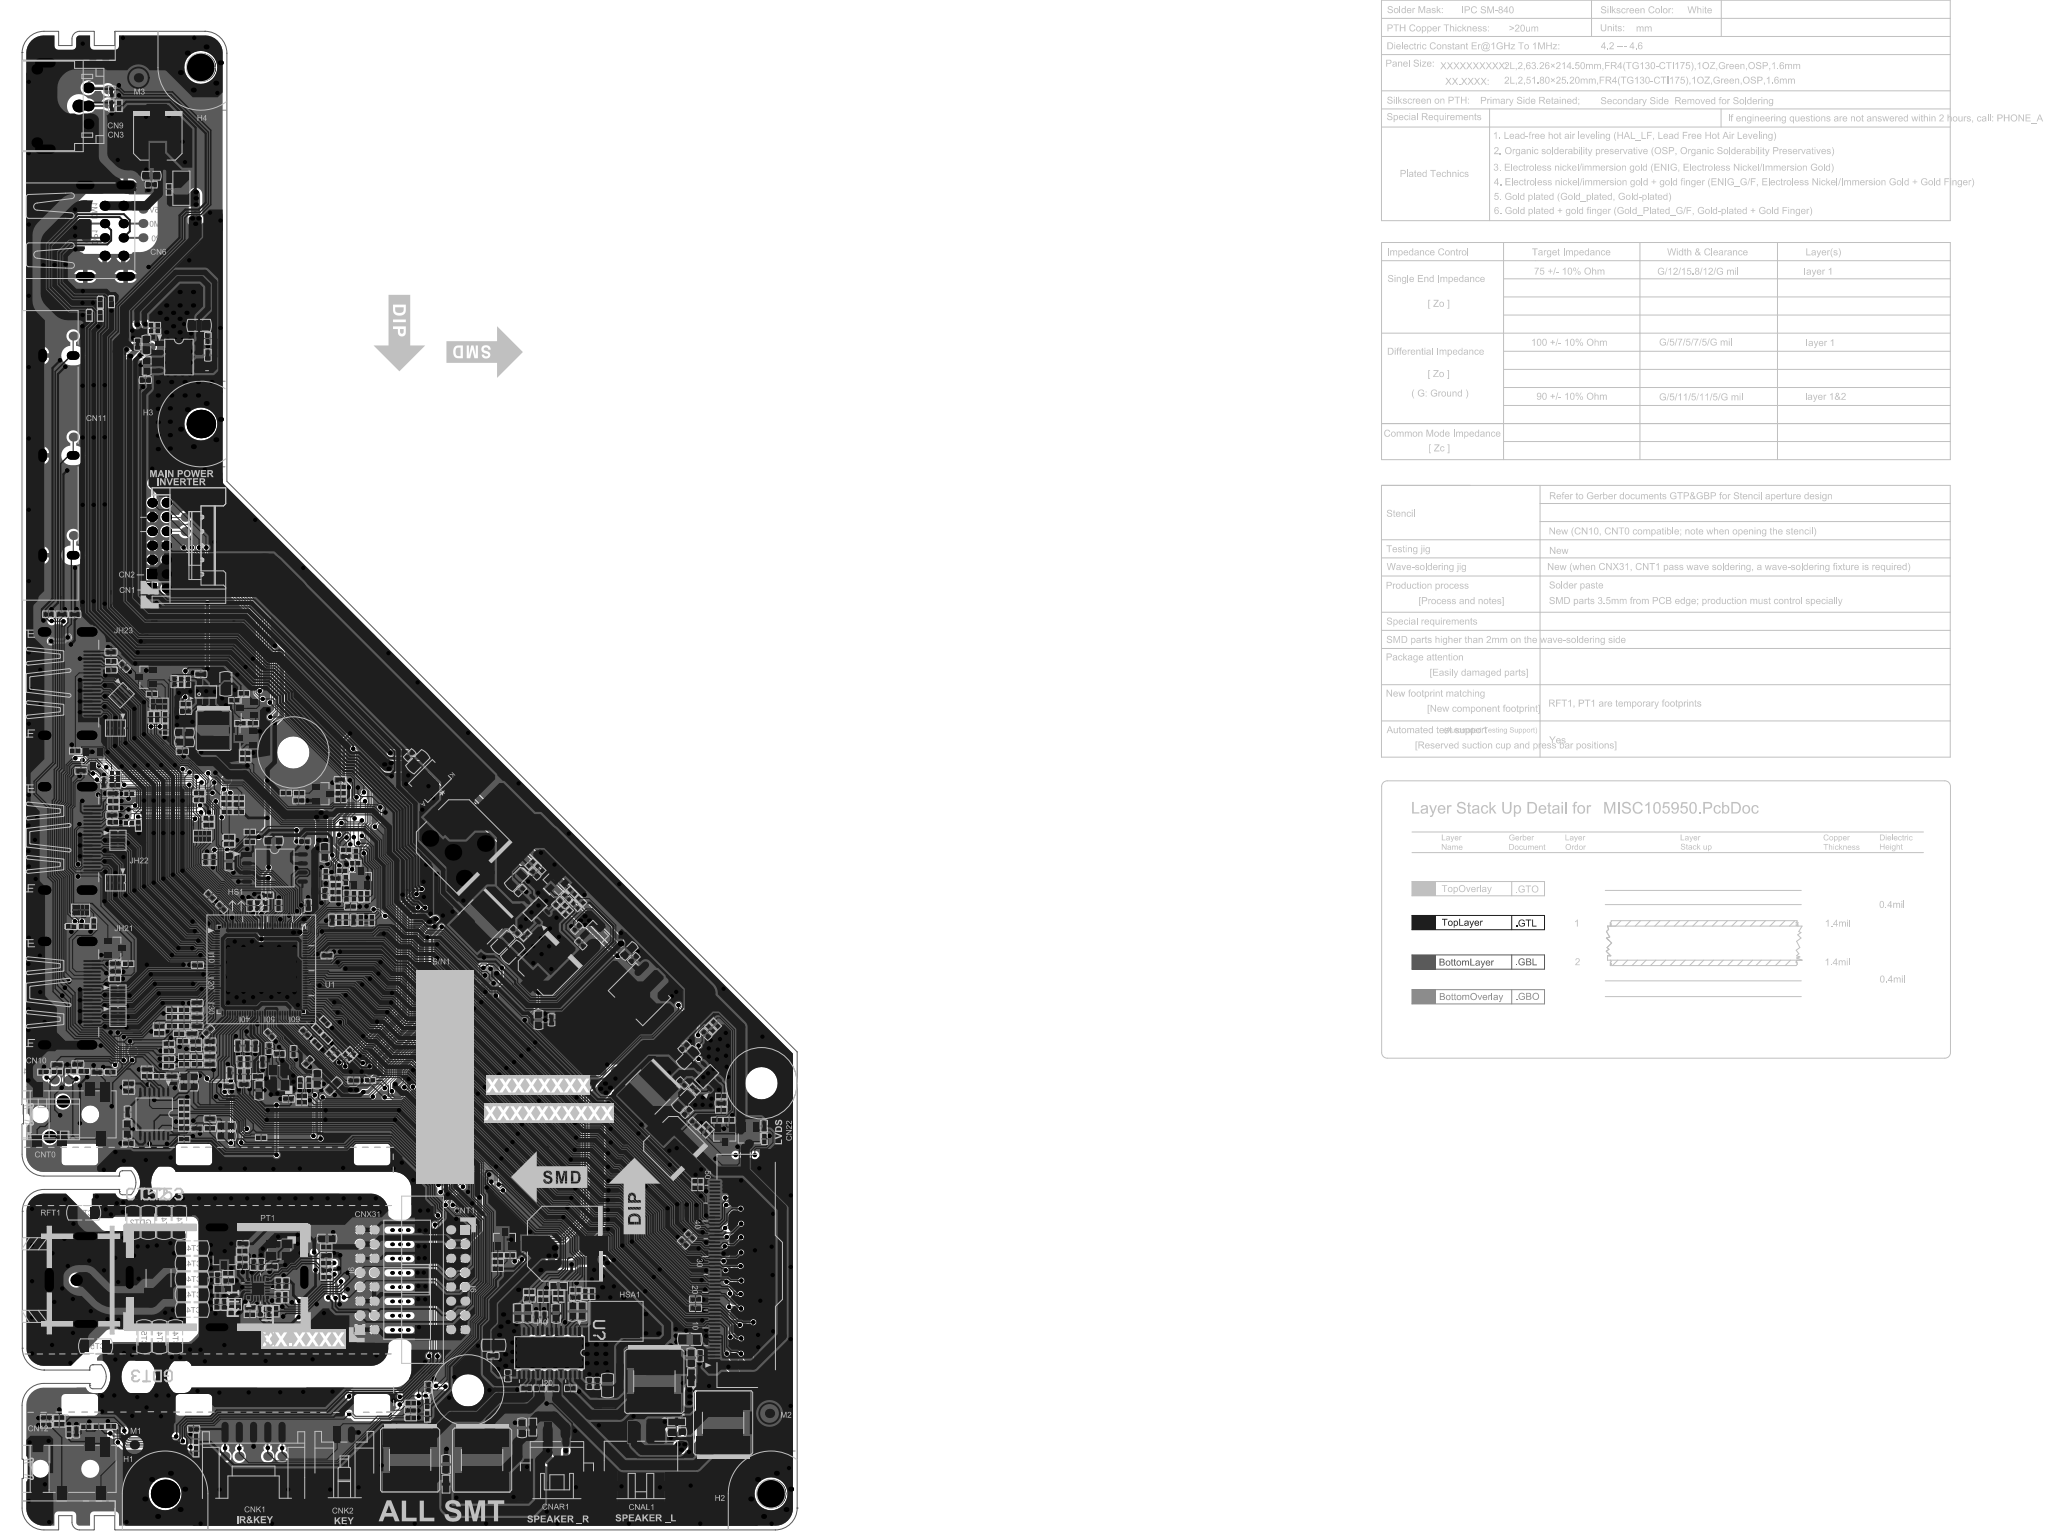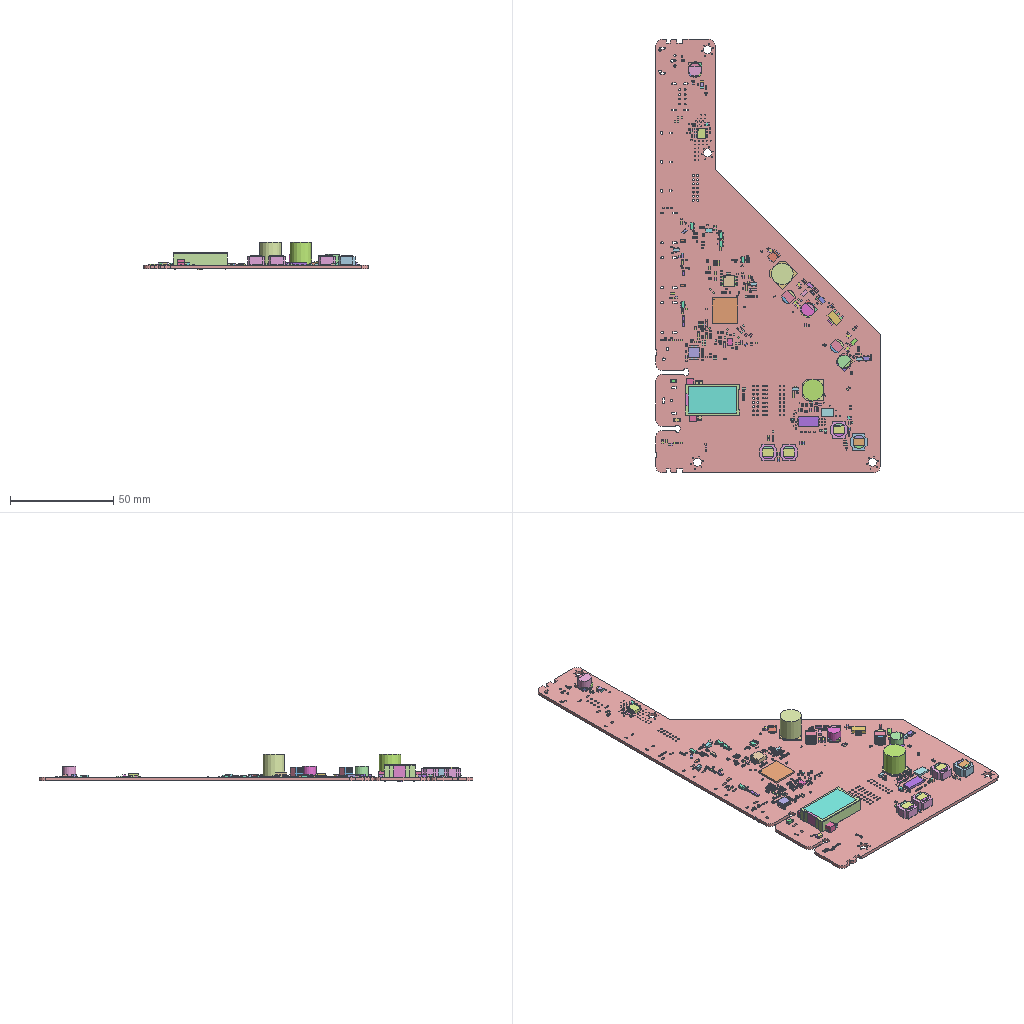Circuit board layout | Altium Designer | box 108.7 x 210.1 x 13.1 mm
Layer stack:
# Altium Designer layer stack of  (unit mm; dielectric type: 0 none, 1 core, 2 prepreg, 3 surface material)
index,name,kind,layer,copper_thickness_mm,dielectric_type,dielectric_thickness_mm,dielectric_material,dielectric_constant
0,TopPaste,other,,,,,,
1,TopOverlay,other,,,,,,
2,TopSolder,dielectric,,,3,0.0102,Solder Resist,3.5
3,TopLayer,copper,TopLayer,0.0356,,,,
4,Dielectric1,dielectric,,,1,1.5,FR-4,4.8
5,BottomLayer,copper,BottomLayer,0.0356,,,,
6,BottomSolder,dielectric,,,3,0.0102,Solder Resist,3.5
7,BottomOverlay,other,,,,,,
8,BottomPaste,other,,,,,,
# drill layer pairs: low layer,high layer
drill_pair,TopLayer,BottomLayer
Part placement, first 366 of 542 lines:
Designator,Comment,Layer,Footprint,Center-X(mm),Center-Y(mm),Rotation
YPbPr_Pb,TEST,BottomLayer,TP,6.464,63.03,180
DI33,NC/SFI0402-240E-2R5PP-LF,TopLayer,DIODE-S0402,20.485,64.935,360
DU31,NC/TVS diode, DIO ESD, 0.1pF, 25V, 0402, SMD, GESD1005H150CR10GPT, Sunlord,TopLayer,DIODE-S0402,41.391,70.115,315
RD66,NC/0ohm-0402-PCB,TopLayer,R0402SC,70.561,83.299,45
RD65,NC/0ohm-0402-PCB,TopLayer,R0402SC,94.272,61.735,315
DU34,NC/TVS diode, DIO ESD, 0.1pF, 25V, 0402, SMD, GESD1005H150CR10GPT, Sunlord,TopLayer,DIODE-S0402,42.596,68.897,135
DU33,NC/TVS diode, DIO ESD, 0.1pF, 25V, 0402, SMD, GESD1005H150CR10GPT, Sunlord,TopLayer,DIODE-S0402,41.262,68.072,135
DU32,NC/TVS diode, DIO ESD, 0.1pF, 25V, 0402, SMD, GESD1005H150CR10GPT, Sunlord,TopLayer,DIODE-S0402,42.481,71.183,315
CK4,NC/NC/0.1uF-0402-X5R-±20%-16V,TopLayer,C0402,56.896,19.926,270
CF59,NC/10uF-0603-X5R-±20%-6.3V,TopLayer,C0603,43.578,62.145,45
CF58,NC/10uF-0603-X5R-±20%-6.3V,TopLayer,C0603,41.339,63.157,90
CF6,NC/10uF-0603-X5R-±20%-6.3V,TopLayer,C0603,33.198,61.587,270
RXD,,BottomLayer,TP,28.575,105.093,270
YPbPr_Y,TEST,BottomLayer,TP,4.464,63.03,180
YPbPr_Pr,TEST,BottomLayer,TP,15.443,67.031,180
YPbPr_GND,TEST,BottomLayer,TP,17.443,67.031,180
ROUT-,DM0,BottomLayer,TP,76.225,9.754,90
ROUT+,DM0,BottomLayer,TP,73.725,9.754,90
LOUT-,DM0,BottomLayer,TP,91.078,14.208,90
LOUT+,DM0,BottomLayer,TP,93.578,14.208,90
GND_AMP,DM0,BottomLayer,TP,88.578,14.208,270
VCC_PANEL1,TEST,BottomLayer,TP,99.784,22.117,90
OCKP,TEST,BottomLayer,TP,99.784,40.117,180
OCKN,TEST,BottomLayer,TP,101.784,40.117,90
O4P,TEST,BottomLayer,TP,99.784,36.117,90
O4N,TEST,BottomLayer,TP,101.784,36.117,180
O3P,TEST,BottomLayer,TP,99.784,38.117,180
O3N,TEST,BottomLayer,TP,101.784,38.117,90
O2P,TEST,BottomLayer,TP,99.784,42.117,180
O2N,TEST,BottomLayer,TP,101.784,42.117,180
O1P,TEST,BottomLayer,TP,99.784,44.117,90
O1N,TEST,BottomLayer,TP,101.784,44.117,180
O0N,TEST,BottomLayer,TP,101.784,46.117,180
GND_TP,TEST,BottomLayer,TP,101.784,22.117,90
ECKP,TEST,BottomLayer,TP,99.784,28.117,180
ECKN,TEST,BottomLayer,TP,101.784,28.117,180
E4P,TEST,BottomLayer,TP,99.784,24.117,180
E4N,TEST,BottomLayer,TP,101.784,24.117,180
E3P,TEST,BottomLayer,TP,99.784,26.117,180
E3N,TEST,BottomLayer,TP,101.784,26.117,180
E2P,TEST,BottomLayer,TP,99.784,30.117,180
E2N,TEST,BottomLayer,TP,101.784,30.117,270
E1P,TEST,BottomLayer,TP,99.784,32.117,180
E1N,TEST,BottomLayer,TP,101.784,32.117,180
E0P,TEST,BottomLayer,TP,99.784,34.117,270
E0N,TEST,BottomLayer,TP,101.784,34.117,180
CT48,NC/Ceramic capacitor, CAP MC, 1KV, 4700pF, ±10%, X7R, 1206, SMD, TP,TopLayer,C1206,21.997,43.053,90
CT47,NC/Ceramic capacitor, CAP MC, 1KV, 4700pF, ±10%, X7R, 1206, SMD, TP,TopLayer,C1206,19.837,43.053,90
CT45,NC/Ceramic capacitor, CAP MC, 1KV, 4700pF, ±10%, X7R, 1206, SMD, TP,TopLayer,C1206,23.801,39.453,360
CT44,Thick-film resistor, RES, 1/4W, 0ohm, ±5%, 1206, SMD,TopLayer,C1206,21.44,27.023,90
CT43,Thick-film resistor, RES, 1/4W, 0ohm, ±5%, 1206, SMD,TopLayer,C1206,23.801,37.283,180
CT42,Thick-film resistor, RES, 1/4W, 0ohm, ±5%, 1206, SMD,TopLayer,C1206,23.801,32.943,180
CT41,Thick-film resistor, RES, 1/4W, 0ohm, ±5%, 1206, SMD,TopLayer,C1206,23.801,30.773,180
UT1,Silicon tuner IC, IC Si Tuner, QFN-24, SMD, ATBM253, AltoBeam,TopLayer,QFN24/0.4-1,33.007,33.782,90
RT5,100ohm-0402-±1%-1/16W,TopLayer,R0402,42.608,37.351,360
RT4,100ohm-0402-±1%-1/16W,TopLayer,R0402,42.634,35.344,360
RT3,33ohm-0402-±1%-1/16W,TopLayer,R0402,36.881,32.563,90
RT2,33ohm-0402-±1%-1/16W,TopLayer,R0402,35.585,30.594,90
LT80,NC/Multilayer inductor, HF Inductor, 270nH, ±5%, 0603, SMD, HCI1608F-R27J-M, Tai-tech,TopLayer,L0603,28.08,33.706,360
LT4,Ferrite bead,BEAD,1000ohm,0402,300mA,SMD,TRAY,CBM100505U102T,FH,TopLayer,L0402,30.289,31.585,90
LT3,Multilayer inductor, HF Inductor, 6.8nH, ±5%, 0402, SMD, MGCI1005T6N8JT-LF, Sunlord,TopLayer,L0402,29.324,31.572,90
LT2,NC/ Multilayer inductor, HF Inductor, 270nH, ±5%, 0402, SMD, SDCL1005CR27JTDF, Sunlord,TopLayer,L0402,28.867,35.89,180
LT1,Thick-film resistor, RES, 1/16W, 0ohm, ±1%, 0402, SMD,TopLayer,L0402,42.608,39.599,180
GDT1,NC/Gas discharge tube, GDT, 700V, 2000A, TP, 4.5×3.2mm, SMD, 4532-091-LF, Brightking,TopLayer,SMD4532-1,19.037,35.255,90
FT2,Ferrite bead,BEAD,1000ohm,0402,300mA,SMD,TRAY,CBM100505U102T,FH,TopLayer,L0402,30.841,39.036,360
DT1,Switching diode,DIO SW D2,200mA,100V,SOT-23,SMD,BAV99,YJ,TopLayer,SO-23,28.283,38.011,360
CT88,0.1uF-0402-X7R-±10%-16V,TopLayer,C0402,30.861,36.929,360
CT77,NC/22pF-0402-NPO-±5%-50V,TopLayer,C0402,35.877,32.55,90
CT61,Ceramic capacitor, CAP MC, 50V, 2pF, ±0.25pF, NPO, 0402, SMD, TP,TopLayer,C0402,28.308,31.56,90
CT49,NC/Ceramic capacitor, CAP MC, 1KV, 4700pF, ±10%, X7R, 1206, SMD, TP,TopLayer,C1206,19.228,27.023,270
CT40,Ceramic capacitor, CAP MC, 1KV, 470pF, ±5%, NPO, 1206, SMD, TP,TopLayer,C1206,23.801,35.112,360
CT29,NC/47pF-0402-NPO-±5%-50V,TopLayer,C0402,42.596,38.367,360
CT28,NC/47pF-0402-NPO-±5%-50V,TopLayer,C0402,42.621,36.36,180
CT21,0.1uF-0402-X7R-±10%-16V,TopLayer,C0402,33.35,30.62,270
CT18,0.1uF-0402-X7R-±10%-16V,TopLayer,C0402,35.877,34.481,90
CT17,NC/Ceramic capacitor, CAP MC, 50V, 1000pF, ±10%, X7R, 0402, SMD, TP,TopLayer,C0402,36.957,34.48,270
CT14,NC/Ceramic capacitor, CAP MC, 50V, 27pF, ±5%, NPO, 0402, SMD, TP,TopLayer,C0402,33.477,37.16,270
CT11,Ceramic capacitor, CAP MC, 50V, 1000pF, ±10%, X7R, 0402, SMD, TP,TopLayer,C0402,30.86,38.008,180
CT7,Thick-film resistor, RES, 1/16W, 0ohm, ±1%, 0402, SMD,TopLayer,C0402,27.241,31.56,90
CT6,NC/22pF-0402-NPO-±5%-50V,TopLayer,C0402,34.582,30.569,90
CT5,NC/0.1uF-0402-X7R-±10%-16V,TopLayer,C0402,30.924,40.056,180
CT4,Thick-film resistor, RES, 1/16W, 0ohm, ±1%, 0402, SMD,TopLayer,C0402,27.369,35.319,90
CT3,0.1uF-0402-X7R-±10%-16V,TopLayer,C0402,32.41,37.16,270
CT2,NC/Ceramic capacitor, CAP MC, 50V, 27pF, ±5%, NPO, 0402, SMD, TP,TopLayer,C0402,34.976,36.855,180
YF11,Passive crystal oscillator, SPXO, 24MHz, ±10ppm, 12pF, SMD3225, SMD, SX32Y024000BC1T-Z, TKD,TopLayer,XTAL-S-3,35.992,39.205,180
PT1,NC/Shield cover, with seal, tinplate, T=0.3mm, natural color, 24.5×14×6mm, JLT,TopLayer,SHIELD(24.5*14*6)-TEMP-NG,27.28,35.357,90
GDT2,NC/Gas discharge tube, GDT, 700V, 2000A, TP, 4.5*3.2mm, SMD, 4532-091-LF, Brightking,TopLayer,SMD4532-1-C1206,16.586,43.053,360
CD54,10uF-0805-X5R-±20%-16V,TopLayer,C0805,28.524,118.566,270
UH22,NC/TVS diode, DIO ESD, 0.4pF, 19V, DFN2510-10L, SMD, ESD5304D-10/TR, Willsemi,TopLayer,RCL0524P,13.03,90.665,180
UH21,NC/TVS diode, DIO ESD, 0.4pF, 19V, DFN2510-10L, SMD, ESD5304D-10/TR, Willsemi,TopLayer,RCL0524P,13.386,96.64,270
CW7,NC/0.1uF-0402-X7R-±10%-16V,TopLayer,C0402,104.026,56.566,90
CW8,0.022uF-0402-X7R-±10%-16V,TopLayer,C0402,94.253,56.946,315
CW9,NC/10uF-0805-X5R-±20%-16V,TopLayer,C0805,93.612,26.645,360
CW10,NC/0.1uF-0402-X7R-±10%-16V,TopLayer,C0402,95.034,24.359,90
QW3,MOSFET, PMOS, -4.3A, -30V, 0.048ohm@ID=-3A@VGS=-4.5V, SOT-23-3L, NCE3407AY, NCEPOWER,TopLayer,SOT-23-1,101.951,55.257,360
QW4,General-purpose transistor, Dynatron, NPN, 0.2A, 40V, 30-300, SOT-23, LMBT3904LT1G, LRC,TopLayer,SOT-23,98.501,55.295,360
RW10,4K7ohm-0402-±1%-1/16W,TopLayer,R0402,96.177,56.375,315
RW11,NC/4K7ohm-0402-±5%-1/16W,TopLayer,R0402,104.076,54.762,270
RW12,47Kohm-0402-±1%-1/16W,TopLayer,R0402,95.549,55.714,135
RW13,4K7ohm-0402-±1%-1/16W,TopLayer,R0402,97.416,57.391,360
RW14,4K7ohm-0402-±1%-1/16W,TopLayer,R0402,99.13,57.391,360
CD39,NC/Ceramic capacitor, CAP MC, 25V, 0.1uF, ±20%, X5R, 0402, SMD, TP,TopLayer,C0402,54.318,108.572,225
CD96,NC/Ceramic capacitor, CAP MC, 25V, 10uF, ±10%, X5R, 0805, SMD, TP,TopLayer,C0805,55.448,107.645,45
DM4,NC/TVS diode, DIO ESD, 26.0V, SMB, SMD, SMBJ16A, GOOD-ARK,TopLayer,DIODE-SMB-2,57.163,104.94,225
EA34,Aluminum electrolytic capacitor, CAP AL, 25V, 470uF, ±20%, LF, RV, 10×10.5, SMD, TP, CapXon,TopLayer,EC(10*10.5)-S,61.227,96.329,45
QD1,General-purpose transistor, Dynatron, PNP, 0.2A, 40V, 30-300, SOT-23, LMBT3906LT1G, LRC,TopLayer,SOT-23,31.516,115.113,270
QD2,General-purpose transistor, Dynatron, NPN, 0.2A, 40V, 30-300, SOT-23, LMBT3904LT1G, LRC,TopLayer,SOT-23,31.343,110.96,270
RD42,510ohm-0402-±1%-1/16W,TopLayer,R0402,31.039,117.221,180
RD43,4K7ohm-0402-±1%-1/16W,TopLayer,R0402,29.725,116.243,360
RD44,10Kohm-0402-±1%-1/16W,TopLayer,R0402,32.291,113.03,180
RD45,NC/0ohm-0402-PCB,TopLayer,R0402SC,30.571,113.03,360
RD46,10Kohm-0402-±1%-1/16W,TopLayer,R0402,31.255,107.975,180
RD47,NC/10Kohm-0402-±5%-1/16W,TopLayer,R0402,31.255,108.89,360
12V/15V,TEST,BottomLayer,TP,83.172,64.275,360
ADJ,TEST,BottomLayer,TP,18.409,146.673,90
BLON,TEST,BottomLayer,TP,20.409,146.673,90
DIM,TEST,BottomLayer,TP,22.82,139.919,180
PWON,TEST,BottomLayer,TP,22.82,141.919,90
1V8_DDR,TEST,BottomLayer,TP,81.172,64.275,270
5V_STB,TEST,BottomLayer,TP,79.172,64.275,180
BG2,General-purpose transistor, Dynatron, NPN, 0.2A, 40V, 30-300, SOT-23, LMBT3904LT1G, LRC,TopLayer,SOT-23,42.152,103.162,90
BG3,NC/General-purpose transistor, Dynatron, NPN, 0.2A, 40V, 30-300, SOT-23, MMBT3904(f=350MHz), BLUE ROCKET,TopLayer,SOT-23,47.409,91.288,180
CD4,NC/0.1uF-0402-X7R-±10%-16V,TopLayer,C0402,92.546,62.585,315
CD7,NC/NC/Ceramic capacitor, CAP MC, 25V, 0.1uF, ±20%, X5R, 0402, SMD, TP,TopLayer,C0402,92.825,67.667,45
CD11,NC/NC/0.1uF-0402-X5R-±20%-16V,TopLayer,C0402,93.205,58.509,225
CD22,NC/0.1uF-0402-X5R-±20%-16V,TopLayer,C0402,25.01,119.926,360
CD24,NC/3300pF-0402-X7R-±10%-50V,TopLayer,C0402,21.285,118.885,270
CD25,10uF-0603-X5R-±20%-6.3V,TopLayer,C0603,22.7,111.747,360
CD26,10uF-0603-X5R-±20%-6.3V,TopLayer,C0603,22.727,110.373,360
CD27,NC/0.1uF-0402-X5R-±20%-16V,TopLayer,C0402,22.407,109.106,360
CD30,Ceramic capacitor, CAP MC, 25V, 10uF, ±10%, X5R, 0805, SMD, TP,TopLayer,C0805,69.291,91.148,225
CD31,NC/Ceramic capacitor, CAP MC, 25V, 0.1uF, ±20%, X5R, 0402, SMD, TP,TopLayer,C0402,69.825,89.599,45
CD50,NC/Ceramic capacitor, CAP MC, 25V, 0.1uF, ±20%, X5R, 0402, SMD, TP,TopLayer,C0402,71.857,91.922,315
CD51,0.1uF-0402-X7R-±10%-16V,TopLayer,C0402,69.126,83.871,315
CD52,Ceramic capacitor, CAP MC, 50V, 1000pF, ±10%, X7R, 0402, SMD, TP,TopLayer,C0402,75.101,87.887,45
CD53,10uF-0805-X5R-±20%-16V,TopLayer,C0805,67.389,82.306,45
CD57,NC/10uF-0805-X5R-±20%-16V,TopLayer,C0805,68.76,80.934,45
CD77,NC/Ceramic capacitor, CAP MC, 25V, 10uF, ±10%, X5R, 0805, SMD, TP,TopLayer,C0805,93.387,66.176,225
CD97,Ceramic capacitor, CAP MC, 6.3V, 1uF, ±20%, X5R, 0402, SMD, TP,TopLayer,C0402,22.88,114.745,180
CD99,NC/10uF-0805-X5R-±20%-16V,TopLayer,C0805,92.716,60.091,45
CG5,NC/0.1uF-0402-X7R-±10%-16V,TopLayer,C0402,38.748,102.21,180
CG6,NC/NC/0.1uF-0402-X7R-±10%-16V,TopLayer,C0402,45.453,88.786,270
CG7,NC/NC/0.1uF-0402-X7R-±10%-16V,TopLayer,C0402,45.364,94.336,360
CG61,NC/0.1uF-0402-X7R-±10%-16V,TopLayer,C0402,44.552,105.118,360
CG66,NC/Ceramic capacitor, CAP MC, 50V, 100pF, ±5%, NPO, 0402, SMD, TP,TopLayer,C0402,43.917,91.313,360
CL11,NC/Ceramic capacitor, CAP MC, 10V, 10uF, ±20%, X5R, 0603, SMD, TP,TopLayer,C0603,85.039,81.102,225
CL12,0.1uF-0402-X7R-±10%-16V,TopLayer,C0402,85.75,80.023,225
CL13,NC/10uF-0603-X5R-±20%-6.3V,TopLayer,C0603,72.377,71.476,270
CL14,1uF-0402-X5R-±20%-6.3V,TopLayer,C0402,74.206,71.45,270
CM1,0.1uF-0402-X7R-±10%-16V,TopLayer,C0402,78.3,82.146,315
CM2,NC/0.1uF-0402-X5R-±20%-16V,TopLayer,C0402,77.762,84.328,45
EA1,Aluminum electrolytic capacitor, CAP AL, 16V, 100uF, ±20%, HV, P, 6.3×5.5, SMD, TP, CapXon,TopLayer,EC(6.5*5.5)-S,73.698,79.058,135
ED6,NC/Aluminum electrolytic capacitor, CAP AL, 16V, 100uF, ±20%, HV, P, 6.3×5.5, SMD, TP, CapXon,TopLayer,EC(6.5*5.5)-S,91.288,53.746,45
LD1,NC/Power inductor, Power Inductor, 4.7uH, ±20%, 2.8A, 0.32×1P, DR5.8×4.5, SMD, PIO54-4R7MTP02, FH,TopLayer,L(5.8*4.5)-S,87.717,61.326,45
LD11,Power inductor, Power Inductor, 4.7uH, ±20%, 2.8A, 0.32×1P, DR5.8×4.5, SMD, PIO54-4R7MTP02, FH,TopLayer,L(5.8*4.5)-S,64.186,85.192,45
LD21,Power inductor, Power Inductor, 2.2uH, ±20%, 2A, 0.28×1P, DR4.5×3.2, SMD, PIO43-2R2MTP02, FH,TopLayer,L(4.5*3.5)-S,26.797,112.052,90
QM1,General-purpose transistor, Dynatron, NPN, 0.2A, 40V, 30-300, SOT-23, LMBT3904LT1G, LRC,TopLayer,SOT-23,75.039,90.935,315
QM2,MOSFET, PMOS, -4.2A, -30V, 0.052ohm@ID=-4.2A@VGS=-10V, SOT-23-3, AO3401, BLUE ROCKET,TopLayer,SOT-23-1,80.012,83.225,135
RD2,100Kohm-0402-±1%-1/16W,TopLayer,R0402,22.867,115.735,360
RD28,NC/4K7ohm-0402-±1%-1/16W,TopLayer,R0402,97.21,70.875,135
RD31,NC/Thick-film resistor, RES, 1/16W, 200Kohm, ±1%, 0402, SMD,TopLayer,R0402,98.014,58.789,180
RD35,NC/Thick-film resistor, RES, 1/16W, 10.5Kohm, ±1%, 0402, SMD,TopLayer,R0402,98.025,60.782,360
RD52,100Kohm-0402-±1%-1/16W,TopLayer,R0402,71.298,93.345,45
RD53,NC/Thick-film resistor, RES, 1/16W, 10Kohm, ±1%, 0402, SMD,TopLayer,R0402,72.581,92.697,315
RD54,Thick-film resistor, RES, 1/16W, 20Kohm, ±1%, 0402, SMD,TopLayer,R0402,76.454,86.512,45
RD81,12Kohm-0402-±1%-1/16W,TopLayer,R0402,22.276,118.872,270
RD88,13Kohm-0402-±1%-1/16W,TopLayer,R0402,23.19,118.872,90
RD91,Thick-film resistor, RES, 1/16W, 150Kohm, ±1%, 0402, SMD,TopLayer,R0402,75.812,87.188,45
RG1,10Kohm-0402-±1%-1/16W,TopLayer,R0402,38.798,103.238,180
RG2,NC/10Kohm-0402-±5%-1/16W,TopLayer,R0402,45.326,91.059,270
RG3,1Kohm-0402-±1%-1/16W,TopLayer,R0402,43.917,90.31,180
RG6,100ohm-0402-±1%-1/16W,TopLayer,R0402,44.615,103.219,180
RG7,NC/100ohm-0402-±5%-1/16W,TopLayer,R0402,46.761,94.755,270
RG8,NC/?,TopLayer,R0402,44.615,104.127,360
RG9,NC/NC/?,TopLayer,R0402,45.377,95.301,360
RG29,4K7ohm-0402-±1%-1/16W,TopLayer,R0402,36.944,103.264,180
RG66,1Kohm-0402-±1%-1/16W,TopLayer,R0402,44.615,102.311,360
RG67,NC/1Kohm-0402-±5%-1/16W,TopLayer,R0402,46.685,93.409,180
RM1,10Kohm-0402-±1%-1/16W,TopLayer,R0402,78.321,88.176,315
RM2,10Kohm-0402-±1%-1/16W,TopLayer,R0402,77.127,89.395,135
RM3,4K7ohm-0402-±1%-1/16W,TopLayer,R0402,76.365,88.659,315
RM4,100Kohm-0402-±1%-1/16W,TopLayer,R0402,77.584,87.452,315
UDA1,NC/DC-DC IC, IC DC-DC, Syn, 2A, 18V, 500kHz, SOT23-6, SMD, SM8102ABC, Silergy,TopLayer,SOT23-6-2,95.974,63.513,45
UDA2,DC-DC IC, IC DC-DC, Syn, 2A, 18V, 500kHz, SOT23-6, SMD, SM8102ABC, Silergy,TopLayer,SOT23-6-2,71.895,86.982,45
UDA3,DC-DC IC, IC DCDC, Syn, 1.2A, 6.0V, 1.5MHz, SOT23-5, SMD, TMI3408, TOLL,TopLayer,SOT-23-5,25.718,117.437,360
UL11,LDO IC, IC LDO, 1A, 1.8V, 15V, SOT-223, SMD, SCJT1117B-1.8V, CJKJ,TopLayer,SOT-223,87.364,75.87,135
VCC_CORE,TEST,BottomLayer,TP,38.57,84.798,315
CNT0,NC/Standoff, F5.5×7.0×7.8mm-M3, nickel-plated, iron, SMT,TopLayer,FIX-5.5*7.0*7.8-S-1,3,57.502,270
CNX31,Connector socket-female, female connect jack, 2×8Pin, D2.0, L, Fool-proofing, Black, L=2.6, DIP, PM-2.0-2*8PW-H=6.35-SK-AC, XFE,TopLayer,SIP2*8H/2.0DF-1,48.325,35.016,90
H3,Location hole,TopLayer,ASSE4.0C-3,24.963,154.85,0
XX.XXXX,PCB_NAME,TopLayer,PCB_NAME,41.275,26.533,90
XXXXXX.,PCB_TIME,TopLayer,PCB_TIME,40.975,26.533,90
3V3_STB,TEST,BottomLayer,TP,15.916,165.789,270
3V3_Tun,TEST,BottomLayer,TP,17.916,165.789,270
5V,DM0,BottomLayer,TP,16.888,185.118,180
AV_CVBS_IN,TEST,BottomLayer,TP,7.099,167.335,180
AV_GND,TEST,BottomLayer,TP,7.112,155.171,180
AV_L_IN,TEST,BottomLayer,TP,7.112,153.171,180
AV_R_IN,TEST,BottomLayer,TP,7.125,139.367,180
CI5,NC/10pF-0402-NPO-±5%-50V,TopLayer,C0402,5.512,128.321,180
CI6,NC/10pF-0402-NPO-±5%-50V,TopLayer,C0402,7.328,128.321,180
CI99,NC/10pF-0402-NPO-±5%-50V,TopLayer,C0402,3.645,128.321,180
CL1,NC/Ceramic capacitor, CAP MC, 10V, 10uF, ±20%, X5R, 0603, SMD, TP,TopLayer,C0603,17.412,163.157,270
CL2,0.1uF-0402-X7R-±10%-16V,TopLayer,C0402,17.221,161.163,360
CL4,Ceramic capacitor, CAP MC, 16V, 1uF, ±20%, X5R, 0402, SMD, TP,TopLayer,C0402,25.997,164.668,90
CL10,NC/10uF-0805-X5R-±20%-16V,TopLayer,C0805,24.765,168.834,180
CL31,NC/Ceramic capacitor, CAP MC, 10V, 10uF, ±20%, X5R, 0603, SMD, TP,TopLayer,C0603,17.372,166.097,90
CL32,0.1uF-0402-X7R-±10%-16V,TopLayer,C0402,16.14,166.199,90
CL34,Ceramic capacitor, CAP MC, 16V, 1uF, ±20%, X5R, 0402, SMD, TP,TopLayer,C0402,25.997,166.992,90
CO22,NC/0.1uF-0402-X5R-±20%-16V,TopLayer,C0402,12.522,201.559,270
CO23,NC/330pF-0402-NPO-±5%-50V,TopLayer,C0402,12.522,199.616,90
COAX,TEST,BottomLayer,TP,11.96,199.863,180
CU1,NC/10uF-0603-X5R-±20%-6.3V,TopLayer,C0603,18.059,189.811,360
CU2,NC/Ceramic capacitor, CAP MC, 16V, 1uF, ±20%, X5R, 0402, SMD, TP,TopLayer,C0402,18.059,188.566,180
DI2,NC/SFI0402-240E-2R5PP-LF,TopLayer,DIODE-S0402,20.498,66.015,360
DI3,NC/SFI0402-240E-2R5PP-LF,TopLayer,DIODE-S0402,43.917,88.43,180
DI22,NC/SFI0402-240E-2R5PP-LF,TopLayer,DIODE-S0402,20.485,67.12,360
DM0,DM0,BottomLayer,TP,16.888,183.118,180
DM1,DM0,BottomLayer,TP,8.917,183.106,270
DP0,DM0,BottomLayer,TP,16.888,181.118,270
DP1,DM0,BottomLayer,TP,8.917,181.106,270
DU1,NC/TVS diode, DIO ESD, 0.1pF, 25V, 0402, SMD, GESD1005H150CR10GPT, Sunlord,TopLayer,DIODE-S0402,12.471,172.12,90
DU2,NC/TVS diode, DIO ESD, 0.1pF, 25V, 0402, SMD, GESD1005H150CR10GPT, Sunlord,TopLayer,DIODE-S0402,10.909,172.044,90
DU11,NC/TVS diode, DIO ESD, 0.1pF, 25V, 0402, SMD, GESD1005H150CR10GPT, Sunlord,TopLayer,DIODE-S0402,10.909,170.215,90
DU12,NC/TVS diode, DIO ESD, 0.1pF, 25V, 0402, SMD, GESD1005H150CR10GPT, Sunlord,TopLayer,DIODE-S0402,9.36,170.215,90
EU1,Aluminum electrolytic capacitor, CAP AL, 16V, 100uF, ±20%, HV, P, 6.3×5.5, SMD, TP, CapXon,TopLayer,EC(6.5*5.5)-S,18.974,195.402,180
FU1,NC/NSMD110(1206-1.1A),TopLayer,FUSE1.1A-S,22.285,188.062,270
RL31,120ohm-0402-±1%-1/16W,TopLayer,R0402,18.021,168.453,90
RL32,200ohm-0402-±1%-1/16W,TopLayer,R0402,18.961,168.453,270
RO31,Thick-film resistor, RES, 1/16W, 0ohm, ±1%, 0402, SMD,TopLayer,R0402,13.564,199.628,270
RU1,Thick-film resistor, RES, 1/16W, 0ohm, ±1%, 0402, SMD,TopLayer,R0402,20.558,187.897,270
SPDIF_OUT,TEST,BottomLayer,TP,11.96,201.863,90
UL1,LDO IC, IC LDO, 1A, 3.3V+ADJ, 12V, ESOP-8, SMD, LC1118CS8TRAD33, Leadchip,TopLayer,SOP8/1.27-3,21.933,164.389,360
DBSR,NO DOLBY,BottomLayer,NO_DOLBY-SILK,-564.783,-896.747,270
XXXXXXXXXX,PCB_NAME,TopLayer,PCB_NAME,227.382,-27.855,90
Manufacture_Info,Manufacture_Info,TopLayer,Manufacture_Info,50.99,74.676,270
M3,MARK,TopLayer,MARK,16.256,203.543,0
M2,MARK,TopLayer,MARK,104.788,16.269,0
M1,MARK,TopLayer,MARK,15.684,11.862,0
CQC,CQC,TopLayer,CQC,-564.783,-896.747,360
XXXXXX,PCB_TIME,TopLayer,PCB_TIME,227.683,-27.855,90
AI_V,AI_GRIPPER_V,TopLayer,AI_GRIPPER_V,129.337,11.176,270
S/N2,Barcode,BottomLayer,Barcode,62.611,63.932,90
S/N1,Barcode,TopLayer,Barcode,59.195,63.462,270
DAS1,35.0*5.4mm,TopLayer,DOLBY_AS2,-564.783,-896.747,90
XXXXXXXX,PCB_NAME,TopLayer,PCB_NAME,228.282,-27.855,90
5V_IR,DM0,BottomLayer,TP,28.385,10.258,90
CA1,Ceramic capacitor, CAP MC, 25V, 10uF, ±10%, X5R, 0805, SMD, TP,TopLayer,C0805,82.067,20.193,270
CA2,NC/Ceramic capacitor, CAP MC, 25V, 10uF, ±10%, X5R, 0805, SMD, TP,TopLayer,C0805,66.078,25.832,180
CA3,3300pF-0402-X7R-±10%-50V,TopLayer,C0402,77.546,32.575,360
CA4,3300pF-0402-X7R-±10%-50V,TopLayer,C0402,71.095,32.34,360
CA5,Ceramic capacitor, CAP MC, 25V, 0.22uF, ±10%, X7R, 0603, SMD, TP,TopLayer,C0603,78.537,30.582,270
CA6,Ceramic capacitor, CAP MC, 25V, 0.22uF, ±10%, X7R, 0603, SMD, TP,TopLayer,C0603,77.165,30.582,270
CA7,Ceramic capacitor, CAP MC, 25V, 1uF, ±10%, X5R, 0603, SMD, TP,TopLayer,C0603,74.854,30.29,90
CA8,1uF-0402-X5R-±20%-16V,TopLayer,C0402,73.199,29.782,270
CA9,NC/1uF-0402-X5R-±20%-16V,TopLayer,C0402,72.071,29.782,270
CA10,Ceramic capacitor, CAP MC, 25V, 0.22uF, ±10%, X7R, 0603, SMD, TP,TopLayer,C0603,70.839,30.315,270
CA11,Ceramic capacitor, CAP MC, 25V, 0.22uF, ±10%, X7R, 0603, SMD, TP,TopLayer,C0603,69.468,30.315,270
CA12,NC/Ceramic capacitor, CAP MC, 25V, 0.1uF, ±20%, X5R, 0402, SMD, TP,TopLayer,C0402,79.515,20.485,270
CA13,1000pF-0402-X7R-±10%-50V,TopLayer,C0402,80.594,20.476,270
CA14,0.22uF-0402-X5R-±10%-16V,TopLayer,C0402,76.886,19.787,180
CA15,0.22uF-0402-X5R-±10%-16V,TopLayer,C0402,74.397,19.787,360
CA17,0.22uF-0402-X5R-±10%-16V,TopLayer,C0402,70.638,19.787,360
CA18,NC/Ceramic capacitor, CAP MC, 25V, 0.1uF, ±20%, X5R, 0402, SMD, TP,TopLayer,C0402,66.002,24.346,180
CA19,1000pF-0402-X7R-±10%-50V,TopLayer,C0402,68.072,21.552,270
CA20,Ceramic capacitor, CAP MC, 25V, 1uF, ±10%, X5R, 0603, SMD, TP,TopLayer,C0603,93.815,24.067,270
CA21,Ceramic capacitor, CAP MC, 25V, 1uF, ±10%, X5R, 0603, SMD, TP,TopLayer,C0603,91.783,13.652,180
CA22,Ceramic capacitor, CAP MC, 25V, 1uF, ±10%, X5R, 0603, SMD, TP,TopLayer,C0603,70.079,14.249,270
CA23,Ceramic capacitor, CAP MC, 25V, 1uF, ±10%, X5R, 0603, SMD, TP,TopLayer,C0603,59.412,9.119,90
CA29,Ceramic capacitor, CAP MC, 6.3V, 22uF, ±20%, X5R, 0603, SMD, TP,TopLayer,C0603,28.6,56.549,360
CA31,NC/NC/Ceramic capacitor, CAP MC, 6.3V, 10uF, ±20%, X5R, 0603, SMD, TP,TopLayer,C0603,23.295,62.103,360
CA32,NC/6800pF-0402-X7R-±10%-50V,TopLayer,C0402,3.34,15.672,180
CA33,NC/6800pF-0402-X7R-±10%-50V,TopLayer,C0402,7.544,13.678,90
CA34,0.22uF-0402-X5R-±10%-16V,TopLayer,C0402,72.53,19.787,180
CA59,NC/NC/Ceramic capacitor, CAP MC, 6.3V, 10uF, ±20%, X5R, 0603, SMD, TP,TopLayer,C0603,28.6,55.188,360
CA60,Ceramic capacitor, CAP MC, 6.3V, 22uF, ±20%, X5R, 0603, SMD, TP,TopLayer,C0603,23.295,63.494,360
CA63,NC/1uF-0402-X5R-±20%-6.3V,TopLayer,C0402,20.949,63.525,180
CA64,NC/1uF-0402-X5R-±20%-6.3V,TopLayer,C0402,26.289,57.556,180
CA65,NC/NC/?,TopLayer,C0402,17.475,64.503,180
CA66,NC/NC/?,TopLayer,C0402,24.453,56.223,180
CA67,NC/1uF-0402-X5R-±20%-6.3V,TopLayer,C0402,14.732,58.522,90
CA68,NC/1uF-0402-X5R-±20%-6.3V,TopLayer,C0402,14.876,62.527,180
CA69,NC/0.1uF-0402-X7R-±10%-16V,TopLayer,C0402,14.876,61.468,180
CA70,NC/Ceramic capacitor, CAP MC, 6.3V, 10uF, ±20%, X5R, 0603, SMD, TP,TopLayer,C0603,14.719,56.131,90
CA71,NC/0.1uF-0402-X5R-±20%-16V,TopLayer,C0402,14.868,54.14,180
CA99,Ceramic capacitor, CAP MC, 6.3V, 1uF, ±20%, X5R, 0402, SMD, TP,TopLayer,C0402,46.465,62.954,180
CD101,NC?,TopLayer,DIODE-S0402,28.981,97.053,180
CD102,NC?,TopLayer,DIODE-S0402,28.981,96.088,180
CF1,20pF-0402-NPO-±5%-50V,TopLayer,C0402,36.008,66.675,180
CF2,0.1uF-0402-X7R-±10%-16V,TopLayer,C0402,39.573,96.469,180
CF3,10uF-0603-X5R-±20%-6.3V,TopLayer,C0603,35.204,96.571,180
CF4,20pF-0402-NPO-±5%-50V,TopLayer,C0402,34.582,67.454,90
CF5,NC/10uF-0603-X5R-±20%-6.3V,TopLayer,C0603,29.02,93.713,90
CF7,0.1uF-0402-X7R-±10%-16V,TopLayer,C0402,32.652,67.771,90
CF8,0.1uF-0402-X7R-±10%-16V,TopLayer,C0402,39.662,69.634,135
CF9,0.1uF-0402-X7R-±10%-16V,TopLayer,C0402,42.71,80.48,180
CF10,0.1uF-0402-X7R-±10%-16V,TopLayer,C0402,34.074,87.486,270
CF11,0.1uF-0402-X7R-±10%-16V,TopLayer,C0402,24.467,73.838,180
CF12,0.1uF-0402-X7R-±10%-16V,TopLayer,C0402,24.524,79.134,360
CF13,0.1uF-0402-X7R-±10%-16V,TopLayer,C0402,26.073,69.901,45
CF14,0.1uF-0402-X7R-±10%-16V,TopLayer,C0402,33.693,65.551,90
CF15,NC/10uF-0603-X5R-±20%-6.3V,TopLayer,C0603,42.367,94.945,90
CF16,0.1uF-0402-X7R-±10%-16V,TopLayer,C0402,40.029,65.569,45
CF17,0.1uF-0402-X7R-±10%-16V,TopLayer,C0402,34.684,69.38,135
CF18,0.1uF-0402-X7R-±10%-16V,TopLayer,C0402,35.916,87.49,90
CF19,0.1uF-0402-X7R-±10%-16V,TopLayer,C0402,40.056,87.528,90
CF20,0.1uF-0402-X7R-±10%-16V,TopLayer,C0402,27.932,87.232,315
CF21,Ceramic capacitor, CAP MC, 6.3V, 1uF, ±20%, X5R, 0402, SMD, TP,TopLayer,C0402,34.345,88.913,180
CF23,Ceramic capacitor, CAP MC, 6.3V, 1uF, ±20%, X5R, 0402, SMD, TP,TopLayer,C0402,38.024,66.993,90
CF24,Ceramic capacitor, CAP MC, 6.3V, 1uF, ±20%, X5R, 0402, SMD, TP,TopLayer,C0402,31.928,87.486,270
CF25,Ceramic capacitor, CAP MC, 6.3V, 2.2uF, ±20%, X5R, 0402, SMD, TP,TopLayer,C0402,33.007,87.486,90
CF26,0.047uF-0402-X7R-±10%-16V,TopLayer,C0402,24.282,68.415,180
CF27,NC/0.1uF-0402-X7R-±10%-16V,TopLayer,C0402,26.289,67.374,360
CF28,1uF-0402-X5R-±20%-6.3V,TopLayer,C0402,26.289,68.44,360
CF29,NC/1000pF-0402-X7R-±10%-50V,TopLayer,C0402,28.943,62.154,360
CF30,NC/1000pF-0402-X7R-±10%-50V,TopLayer,C0402,29.07,64.014,90
CF70,0.047uF-0402-X7R-±10%-16V,TopLayer,C0402,19.177,70.561,180
CF71,NC/5pF-0402-NPO-±5%-50V,TopLayer,C0402,94.399,31.026,180
CF90,NC/1000pF-0402-X7R-±10%-50V,TopLayer,C0402,37.312,60.376,180
CF94,NC/5pF-0402-NPO-±5%-50V,TopLayer,C0402,94.399,32.263,180
CF95,NC/5.6pF-0402-NPO-±5%-50V,TopLayer,C0402,92.732,40.183,135
CF96,NC/5.6pF-0402-NPO-±5%-50V,TopLayer,C0402,93.691,41.135,135
CH1,NC/0.1uF-0402-X7R-±10%-16V,TopLayer,C0402,13.018,78.257,360
CH2,NC/0.1uF-0402-X7R-±10%-16V,TopLayer,C0402,13.017,79.324,180
CH3,NC/?,TopLayer,C0402,43.421,85.433,270
CH21,NC/0.1uF-0402-X7R-±10%-16V,TopLayer,C0402,12.709,103.177,180
CH22,NC/0.1uF-0402-X7R-±10%-16V,TopLayer,C0402,11.417,104.686,90
CH60,NC/?,TopLayer,C0402,46.444,85.458,270
CH70,NC/0.1uF-0402-X7R-±10%-16V,TopLayer,C0402,14.262,121.031,315
CH71,NC/0.1uF-0402-X7R-±10%-16V,TopLayer,C0402,12.408,123.025,360
CH72,NC/?,TopLayer,C0402,25.692,93.939,270
CH81,Ceramic capacitor, CAP MC, 6.3V, 1uF, ±20%, X5R, 0402, SMD, TP,TopLayer,C0402,26.34,88.824,315
CH101,NC/10pF-0402-NPO-±5%-50V,TopLayer,C0402,8.195,106.362,360
CH102,NC/10pF-0402-NPO-±5%-50V,TopLayer,C0402,12.543,100.168,180
CI3,1uF-0402-X5R-±20%-6.3V,TopLayer,C0402,26.289,66.294,180
CI4,1uF-0402-X5R-±20%-6.3V,TopLayer,C0402,26.289,65.227,180
CI33,0.047uF-0402-X7R-±10%-16V,TopLayer,C0402,23.762,69.507,360
CI70,NC/10pF-0402-NPO-±5%-50V,TopLayer,C0402,7.747,65.24,360
CI71,NC/10pF-0402-NPO-±5%-50V,TopLayer,C0402,10.439,64.122,360
CI72,NC/10pF-0402-NPO-±5%-50V,TopLayer,C0402,4.839,65.126,180
CI93,0.047uF-0402-X7R-±10%-16V,TopLayer,C0402,24.473,70.574,360
CI95,0.047uF-0402-X7R-±10%-16V,TopLayer,C0402,24.473,72.873,360
CI98,0.047uF-0402-X7R-±10%-16V,TopLayer,C0402,24.473,71.819,360
CK1,Ceramic capacitor, CAP MC, 50V, 470pF, ±5%, NPO, 0402, SMD, TP,TopLayer,C0402,42.418,89.179,270
CK3,0.1uF-0402-X7R-±10%-16V,TopLayer,C0402,24.003,14.084,180
CK5,NC/0.1uF-0402-X7R-±10%-16V,TopLayer,C0402,54.432,16.675,180
CK11,0.01uF-0402-X7R-±10%-50V,TopLayer,C0402,26.759,93.939,270
CN1,连接插座,connect jack,2×7PIN,D2.0,L,SNAP,STEP,Fool-proofing,Nature,L=2.5,SMD,PHD-2*7AW-DK-SMT-P,XFE,TopLayer,SIP2*7H/2.0D-LS,18.952,137.956,90
CN2,NC/Connector socket, connect jack, 2×6PIN, D2.0, L, SNAP, STEP, Fool-proofing, Nature, L=2.5, SMD, PHD-2*6AW-DK-SMT-P, XFE-D,TopLayer,SIP2*6H/2.0D-LS,18.952,138.956,90
CN3,NC/RCA jack, RCA Jack, AV1, H, Orange, CH5.5, Seal, SMD, RCA-143P1-EP-07, CS,TopLayer,AV1-H-4-S,5.55,199.587,270
CN6,USB jack, USB Receptacle, USB2.0, H, Double, Black, flange, Block up, SMD, WLUS-392A, WLCO,TopLayer,USB2-HS-1,11.746,182.1,270
CN9,Optical jack, OPTICAL, H, SMD, 182500122, VAST,TopLayer,OPTICAL-HS-1,5.6,199.6,270
CN10,Earphone jack, Earphone Jack, H, F3.5, CH2.25, Black, switch, Seal, SMD, PJ-342F, JSL,TopLayer,PHONE-HS-29,6.825,58.125,270
CN11,RCA jack, RCA Jack, AV3, H, Yellow, White, Red, CH5.5, D14, Seal, SMD, AV3-8.4-18A, JSL,TopLayer,AV3-H14-15-S,4.95,150.6,270
CN22,FFC connector, FFC connector, 51Pin, D0.5, Bottom, lock, SMD, CT,TopLayer,FFC51H/0.5S-8,100.79,36.255,90
CNAL1,Connector socket, connect jack, 2pin, D2.5, L, SNAP, Fool-proofing, Nature, L=2.4mm, SMD, AMA,TopLayer,SIP2H/2.5S-4,86.754,9.87,0
CNAR1,Connector socket, 2PIN, D2.5, L, SNAP, Fool-proofing, RED, SMD, XFE,TopLayer,SIP2H/2.5S-3,74.968,9.668,0
CNK1,Connector socket, connect jack, 5pin, D2.0, L, SNAP, STEP, Fool-proofing, Nature, L=2.5mm, SMD, AMA,TopLayer,SIP5H/2.0S-4,32.408,9.602,360
CNK2,Connector socket, Connect jack, 2Pin, D2.0, L, SNAP, STEP, Fool-proofing, Nature, L=2.5mm, SMD, S2015-02R2WA-KSY, XYDT,TopLayer,SIP2H/2.0S-3,45.141,9.602,0
CO21,NC/33pF-0402-NPO-±5%-50V,TopLayer,C0402,45.999,87.338,180
CT1,0.1uF-0402-X7R-±10%-16V,TopLayer,C0402,30.518,65.576,270
CT8,NC/47pF-0402-NPO-±5%-50V,TopLayer,C0402,30.201,67.805,90
CT9,NC/0.1uF-0402-X7R-±10%-16V,TopLayer,C0402,31.073,62.408,180
CT10,NC/47pF-0402-NPO-±5%-50V,TopLayer,C0402,31.521,67.805,270
CT12,0.1uF-0402-X7R-±10%-16V,TopLayer,C0402,31.598,65.576,270
Pad and via stacks, first 77 of 153 lines:
# Altium Designer via and pad stacks of  (unit mm). Each distinct definition once, with the count of objects using it.
# via: kind,start_layer,end_layer,hole_mm,diameter_mm,mode(0 simple;1 top-mid-bottom;2 full stack),diameter_per_layer,count,example_net
# pad: kind,layer,hole_mm,hole_type(0 round;1 square;2 slot),plating,top_size,top_shape(1 round;2 rect;3 octagon;9 rounded rect),mid_size,bottom_size,mode,footprint,size_per_layer,count,example
pad,TopOverlay,0,0,plated,1.3x1.3,2,1.3x1.3,1.3x1.3,0,SIP2*8H/2.0DM-1,,1,CNT1.0
pad,TopOverlay,0,0,plated,1.3x1.3,1,1.3x1.3,1.3x1.3,0,SIP2*8H/2.0DM-1,,15,CNT1.0
pad,TopOverlay,0,0,plated,1.3x1.3,2,1.3x1.3,1.3x1.3,0,SIP2*8H/2.0DF-1,,1,CNX31.0
pad,TopOverlay,0,0,plated,1.3x1.3,1,1.3x1.3,1.3x1.3,0,SIP2*8H/2.0DF-1,,15,CNX31.0
pad,TopLayer,0,0,plated,0.5x0.45,2,0.5x0.45,0.5x0.45,0,R0402,,238,RF19.2
pad,TopLayer,0,0,plated,0.5x0.45,9,0.5x0.45,0.5x0.45,0,C0402,,280,CF70.2
pad,TopLayer,0,0,plated,0.3x0.3,2,0.3x0.3,0.3x0.3,0,C0402,,280,CF70.1
pad,TopLayer,0,0,plated,0.8x0.8,2,0.8x0.8,0.8x0.8,0,C0603,,56,CA59.1
pad,TopLayer,0,0,plated,0.25x0.42,2,0.25x0.42,0.25x0.42,0,R0402SC,,11,R99.3
pad,TopLayer,0,0,plated,0.5x0.45,2,0.5x0.45,0.5x0.45,0,R0402SC,,24,R99.2
pad,TopLayer,0,0,plated,0.55x0.45,2,0.55x0.45,0.55x0.45,0,DIODE-S0402,,80,DU31.A
pad,TopLayer,0,0,plated,0.22x0.7,1,0.22x0.7,0.22x0.7,0,QFN128/0.35-1,,127,U1.128
pad,TopLayer,0,0,plated,0.22x0.7,2,0.22x0.7,0.22x0.7,0,QFN128/0.35-1,,1,U1.1
pad,TopLayer,0,0,unplated,6.3x9.6,2,6.3x9.6,6.3x9.6,0,QFN128/0.35-1,,1,U1.EPAD
pad,TopLayer,0,0,plated,2.75x1.4,2,2.75x1.4,2.75x1.4,0,PHONE-HS-29,,2,CN10.6
pad,TopLayer,0,0,plated,1.9x1.4,2,1.9x1.4,1.9x1.4,0,PHONE-HS-29,,2,CN10.4
pad,TopLayer,0,0,plated,2.1x1.4,2,2.1x1.4,2.1x1.4,0,PHONE-HS-29,,6,CN10.5
pad,TopLayer,0,0,plated,1.6x1.4,2,1.6x1.4,1.6x1.4,0,PHONE-HS-29,,2,CN10.1
pad,TopLayer,0,0,plated,0.8x0.21,2,0.8x0.21,0.8x0.21,0,RCL0524P,,6,UH2.1
pad,TopLayer,0,0,plated,0.8x0.21,1,0.8x0.21,0.8x0.21,0,RCL0524P,,42,UH2.5
pad,TopLayer,0,0,plated,0.8x0.38,2,0.8x0.38,0.8x0.38,0,RCL0524P,,12,UH2.GND
pad,TopLayer,0,0,plated,0.26x2.5,1,0.26x2.5,0.26x2.5,0,HDMI-HS-1,,57,JH21.2
pad,TopLayer,0,0,plated,0.8x1.1,2,0.8x1.1,0.8x1.1,0,SOT-23,,10,QD1.C
pad,TopLayer,0,0,plated,0.8x1,2,0.8x1,0.8x1,0,SOT-23,,20,QD1.E
pad,TopLayer,0,0,plated,0.5x0.5,2,0.5x0.5,0.5x0.5,0,RA0402,,16,RH24.8
pad,TopLayer,0,0,plated,0.5x0.3,2,0.5x0.3,0.5x0.3,0,RA0402,,16,RH24.4
pad,TopLayer,0,0,plated,1.4x1.1,2,1.4x1.1,1.4x1.1,0,XTAL-S-3,,8,YF1.2
pad,TopLayer,0,0,plated,0.3x1.225,1,0.3x1.225,0.3x1.225,0,SSOP14/0.65-1,,14,UA61.3
pad,TopLayer,0,0,plated,0.1778x0.66,2,0.1778x0.66,0.1778x0.66,0,GND,,6,RA65.JP_1K
pad,TopLayer,0,0,plated,0.3048x0.42,2,0.3048x0.42,0.3048x0.42,0,R0402SC,,1,R9.3
pad,TopLayer,0,0,plated,1.5x0.6,1,1.5x0.6,1.5x0.6,0,SOIC8,,7,UF1.8
pad,TopLayer,0,0,plated,1.5x0.6,2,1.5x0.6,1.5x0.6,0,SOIC8,,1,UF1.1
pad,TopLayer,0,0,plated,0.3x0.66,2,0.3x0.66,0.3x0.66,0,GND,,2,RA64.JP_1K
pad,TopLayer,0,0,plated,0.6x0.8,2,0.6x0.8,0.6x0.8,0,SOT-23-5,,5,UDA3.4
pad,TopLayer,0,0,plated,4.3x1.8,2,4.3x1.8,4.3x1.8,0,L(4.5*3.5)-S,,2,LD21.2
pad,TopLayer,0,0,plated,5.5x2.5,2,5.5x2.5,5.5x2.5,0,L(5.8*4.5)-S,,4,LD11.2
pad,TopLayer,0,0,plated,3.85x2,2,3.85x2,3.85x2,0,EC(10*10.5)-S,,4,EA34.1
pad,TopLayer,0,0,plated,1.6x2.2,2,1.6x2.2,1.6x2.2,0,DIODE-SMB-2,,2,DM4.A
pad,TopLayer,0,0,plated,1.25x0.9,2,1.25x0.9,1.25x0.9,0,C0805,,22,CD96.2
pad,TopLayer,0,0,plated,1.238x0.6,1,1.238x0.6,1.238x0.6,0,SOP8/1.27-3,,7,UL1.8
pad,TopLayer,0,0,plated,1.238x0.6,2,1.238x0.6,1.238x0.6,0,SOP8/1.27-3,,1,UL1.1
pad,TopLayer,0,0,plated,3.5x5,2,3.5x5,3.5x5,0,SOP8/1.27-3,,1,UL1.EPAD
pad,TopLayer,0,0,plated,1.3x1.3,1,1.3x1.3,1.3x1.3,0,MARK,,3,M3.0
pad,TopLayer,0,0,plated,2x1,2,2x1,2x1,0,FUSE1.1A-S,,2,FU1.1
pad,TopLayer,0,0,plated,3.5x2,2,3.5x2,3.5x2,0,EC(6.5*5.5)-S,,6,EU1.1
pad,TopLayer,0,0,plated,2x2,2,2x2,2x2,0,,,17,HS60
pad,TopLayer,0,0,plated,4x2.5,2,4x2.5,4x2.5,0,SOT-223,,1,UL11.4
pad,TopLayer,0,0,plated,1x2.5,1,1x2.5,1x2.5,0,SOT-223,,3,UL11.1
pad,TopLayer,0,0,plated,0.5x1,1,0.5x1,0.5x1,0,SOT23-6-2,,12,UDA2.2
pad,TopLayer,0,0,plated,0.8x1.1,2,0.8x1.1,0.8x1.1,0,SOT-23-1,,2,QM2.D
pad,TopLayer,0,0,plated,0.8x1.27,2,0.8x1.27,0.8x1.27,0,SOT-23-1,,4,QM2.G
pad,TopLayer,0,0,plated,1x1.6,2,1x1.6,1x1.6,0,C1206,,28,CT51.2
pad,TopLayer,0,0,plated,1x0.82,2,1x0.82,1x0.82,0,R0603SC,,4,RA22.3
pad,TopLayer,0,0,plated,0.8x0.7,2,0.8x0.7,0.8x0.7,0,R0603SC,,8,RA22.2
pad,TopLayer,0,0,plated,0.55x0.45,2,0.55x0.45,0.55x0.45,0,L0402,,10,FT2.1
pad,TopLayer,0,0,plated,1.5x4,2,1.5x4,1.5x4,0,SMD4532-1,,2,GDT1.2
pad,TopLayer,0,0,plated,0.8x0.8128,2,0.8x0.8128,0.8x0.8128,0,L0603,,2,LT80.1
pad,TopLayer,0,0,plated,1x3,1,1x3,1x3,0,SIP5H/2.0S-4,,5,CNK1.4
pad,TopLayer,0,0,plated,1.5x3,2,1.5x3,1.5x3,0,SIP5H/2.0S-4,,2,CNK1.7
pad,TopLayer,0,0,plated,1.8x3.9,2,1.8x3.9,1.8x3.9,0,SIP2H/2.5S-3,,2,CNAR1.4
pad,TopLayer,0,0,plated,1x3.5,2,1x3.5,1x3.5,0,SIP2H/2.5S-3,,1,CNAR1.1
pad,TopLayer,0,0,plated,1x3.5,1,1x3.5,1x3.5,0,SIP2H/2.5S-3,,1,CNAR1.2
pad,TopLayer,0,0,plated,2.1x3.9,2,2.1x3.9,2.1x3.9,0,SIP2H/2.5S-4,,2,CNAL1.3
pad,TopLayer,0,0,plated,1x3,1,1x3,1x3,0,SIP2H/2.5S-4,,1,CNAL1.2
pad,TopLayer,0,0,plated,1x3,2,1x3,1x3,0,SIP2H/2.5S-4,,1,CNAL1.1
pad,TopLayer,0,0,unplated,6.6x4.6,2,6.6x4.6,6.6x4.6,0,HL030,,1,HSA1.1
pad,TopLayer,0,0,plated,1.55x0.25,1,1.55x0.25,1.55x0.25,0,FFC51H/0.5S-8,,51,CN22.51
pad,TopLayer,0,0,plated,2.1x1.6,2,2.1x1.6,2.1x1.6,0,FFC51H/0.5S-8,,2,CN22.52
pad,TopLayer,0,0,plated,7.5x2.4,2,7.5x2.4,7.5x2.4,0,L(8*4.2)-S,,8,LA3.2
pad,TopLayer,0,0,plated,5.5x2.5,2,5.5x2.5,5.5x2.5,0,L(5.8*4.5)-S-3,,8,LA2.S
pad,TopLayer,0,0,plated,1.5x3.6,2,1.5x3.6,1.5x3.6,0,SIP2H/2.0S-3,,2,CNK2.3
pad,TopLayer,0,0,plated,1x2.3,1,1x2.3,1x2.3,0,SIP2H/2.0S-3,,1,CNK2.2
pad,TopLayer,0,0,plated,1x2.3,2,1x2.3,1x2.3,0,SIP2H/2.0S-3,,1,CNK2.1
pad,TopLayer,0,0,plated,0.8x1.1,2,0.8x1.1,0.8x1.1,0,SO-23,,1,DT1.2
Copper pours:
name,layer,net,type(0 solid;1 hatched;2 none)
5,BottomLayer,GND,0
5,BottomLayer,GND,0
12,BottomLayer,RFGND,0
12,BottomLayer,GND,0
12,BottomLayer,GND,0
5,BottomLayer,GND,0
12,TopLayer,GND,0
12,TopLayer,RFGND,0
5,TopLayer,GND,0
5,TopLayer,GND,0
5,TopLayer,GND,0
Design rules, without the lines most boards share, first 19 of 31 lines:
# Altium Designer design rules of  (exported by Altium Designer, unit mm)
# columns: name | kind | enabled | priority | scope1 | scope2 | descriptor | typed fields (field=value)
NetAntennae | 56 | enabled | 1 | Not (HasFootprint('ANT-7') or HasFootprint('ANT-BLUECORE')) | All | Net Antennae (Tolerance=40mil) (Not (HasFootprint('ANT-7') or HasFootprint('ANT-BLUECORE'))) |
Hole2Hole | 52 | disabled | 1 | All | All | Hole To Hole Clearance (Gap=18mil) (Disabled)(All),(All) | gap=0.4572
DiffPairsRouting | 51 | enabled | 4 | All | All | Differential Pairs Uncoupled Length using the Gap Constraints (Min=10mil) (Max=10mil) (Prefered=10mil)  and Width Constraints (Min=15mil) (Max=15mil) (Prefered=15mil) (All) |
TestPointUsage | 44 | enabled | 1 | All | All | Fabrication Testpoint Usage (Valid =One Required, Allow multiple per net=No) (All) |
Testpoint | 43 | enabled | 1 | All | All | Fabrication Testpoint Style (Under Component=Yes) (All) |
HoleSize_VIA | 42 | disabled | 1 | ISVIA | All | Hole Size Constraint (Min=7.874mil) (Max=23.622mil) (Disabled)(ISVIA) |
PermittedLayers | 26 | enabled | 1 | All | All | Permitted Layers - (Top Layer, Bottom Layer) (All) |
SMDToCorner | 23 | disabled | 1 | All | All | SMD To Corner (Distance=4mil) (Disabled)(All) |
MinimumAnnularRing | 19 | enabled | 1 | All | All | Minimum Annular Ring (Minimum=3.937mil) (All) |
ViasUnderSMD | 17 | enabled | 1 | All | All | Vias Under SMD Constraint (Allowed=Not Allowed) (All) |
PasteMaskExpansion | 14 | enabled | 1 | All | All | Paste Mask Expansion (Expansion =0mil) (All) | expansion=0
0.25_0.1 | 11 | disabled | 6 | All | All | Routing Via (MinHoleWidth=3.937mil) (MaxHoleWidth=3.937mil) (PreferredHoleWidth=3.937mil) (MinWidth=9.842mil) (MaxWidth=9.842mil) (PreferedWidth=9.842mil) (Disabled)(All) | via_min_hole=0.1 via_max_hole=0.1 via_preferred_diameter=0.25 via_preferred_hole=0.1
0.4_0.2 | 11 | disabled | 5 | All | All | Routing Via (MinHoleWidth=7.874mil) (MaxHoleWidth=7.874mil) (PreferredHoleWidth=7.874mil) (MinWidth=15.748mil) (MaxWidth=15.748mil) (PreferedWidth=15.748mil) (Disabled)(All) | via_min_hole=0.2 via_max_hole=0.2 via_preferred_diameter=0.4 via_preferred_hole=0.2
0.45_0.25 | 11 | disabled | 4 | All | All | Routing Via (MinHoleWidth=9.842mil) (MaxHoleWidth=9.842mil) (PreferredHoleWidth=9.842mil) (MinWidth=17.716mil) (MaxWidth=17.716mil) (PreferedWidth=17.716mil) (Disabled)(All) | via_min_hole=0.25 via_max_hole=0.25 via_preferred_diameter=0.45 via_preferred_hole=0.25
0.5_0.3 | 11 | disabled | 3 | All | All | Routing Via (MinHoleWidth=11.811mil) (MaxHoleWidth=11.811mil) (PreferredHoleWidth=11.811mil) (MinWidth=19.685mil) (MaxWidth=19.685mil) (PreferedWidth=19.685mil) (Disabled)(All) | via_min_hole=0.3 via_max_hole=0.3 via_preferred_diameter=0.5 via_preferred_hole=0.3
0.8_0.5 | 11 | disabled | 2 | All | All | Routing Via (MinHoleWidth=19.685mil) (MaxHoleWidth=19.685mil) (PreferredHoleWidth=19.685mil) (MinWidth=31.496mil) (MaxWidth=31.496mil) (PreferedWidth=31.496mil) (Disabled)(All) | via_min_hole=0.5 via_max_hole=0.5 via_preferred_diameter=0.8 via_preferred_hole=0.5
0.6_0.4 | 11 | enabled | 1 | All | All | Routing Via (MinHoleWidth=15.748mil) (MaxHoleWidth=15.748mil) (PreferredHoleWidth=15.748mil) (MinWidth=23.622mil) (MaxWidth=23.622mil) (PreferedWidth=23.622mil) (All) | via_min_hole=0.4 via_max_hole=0.4 via_preferred_diameter=0.6 via_preferred_hole=0.4